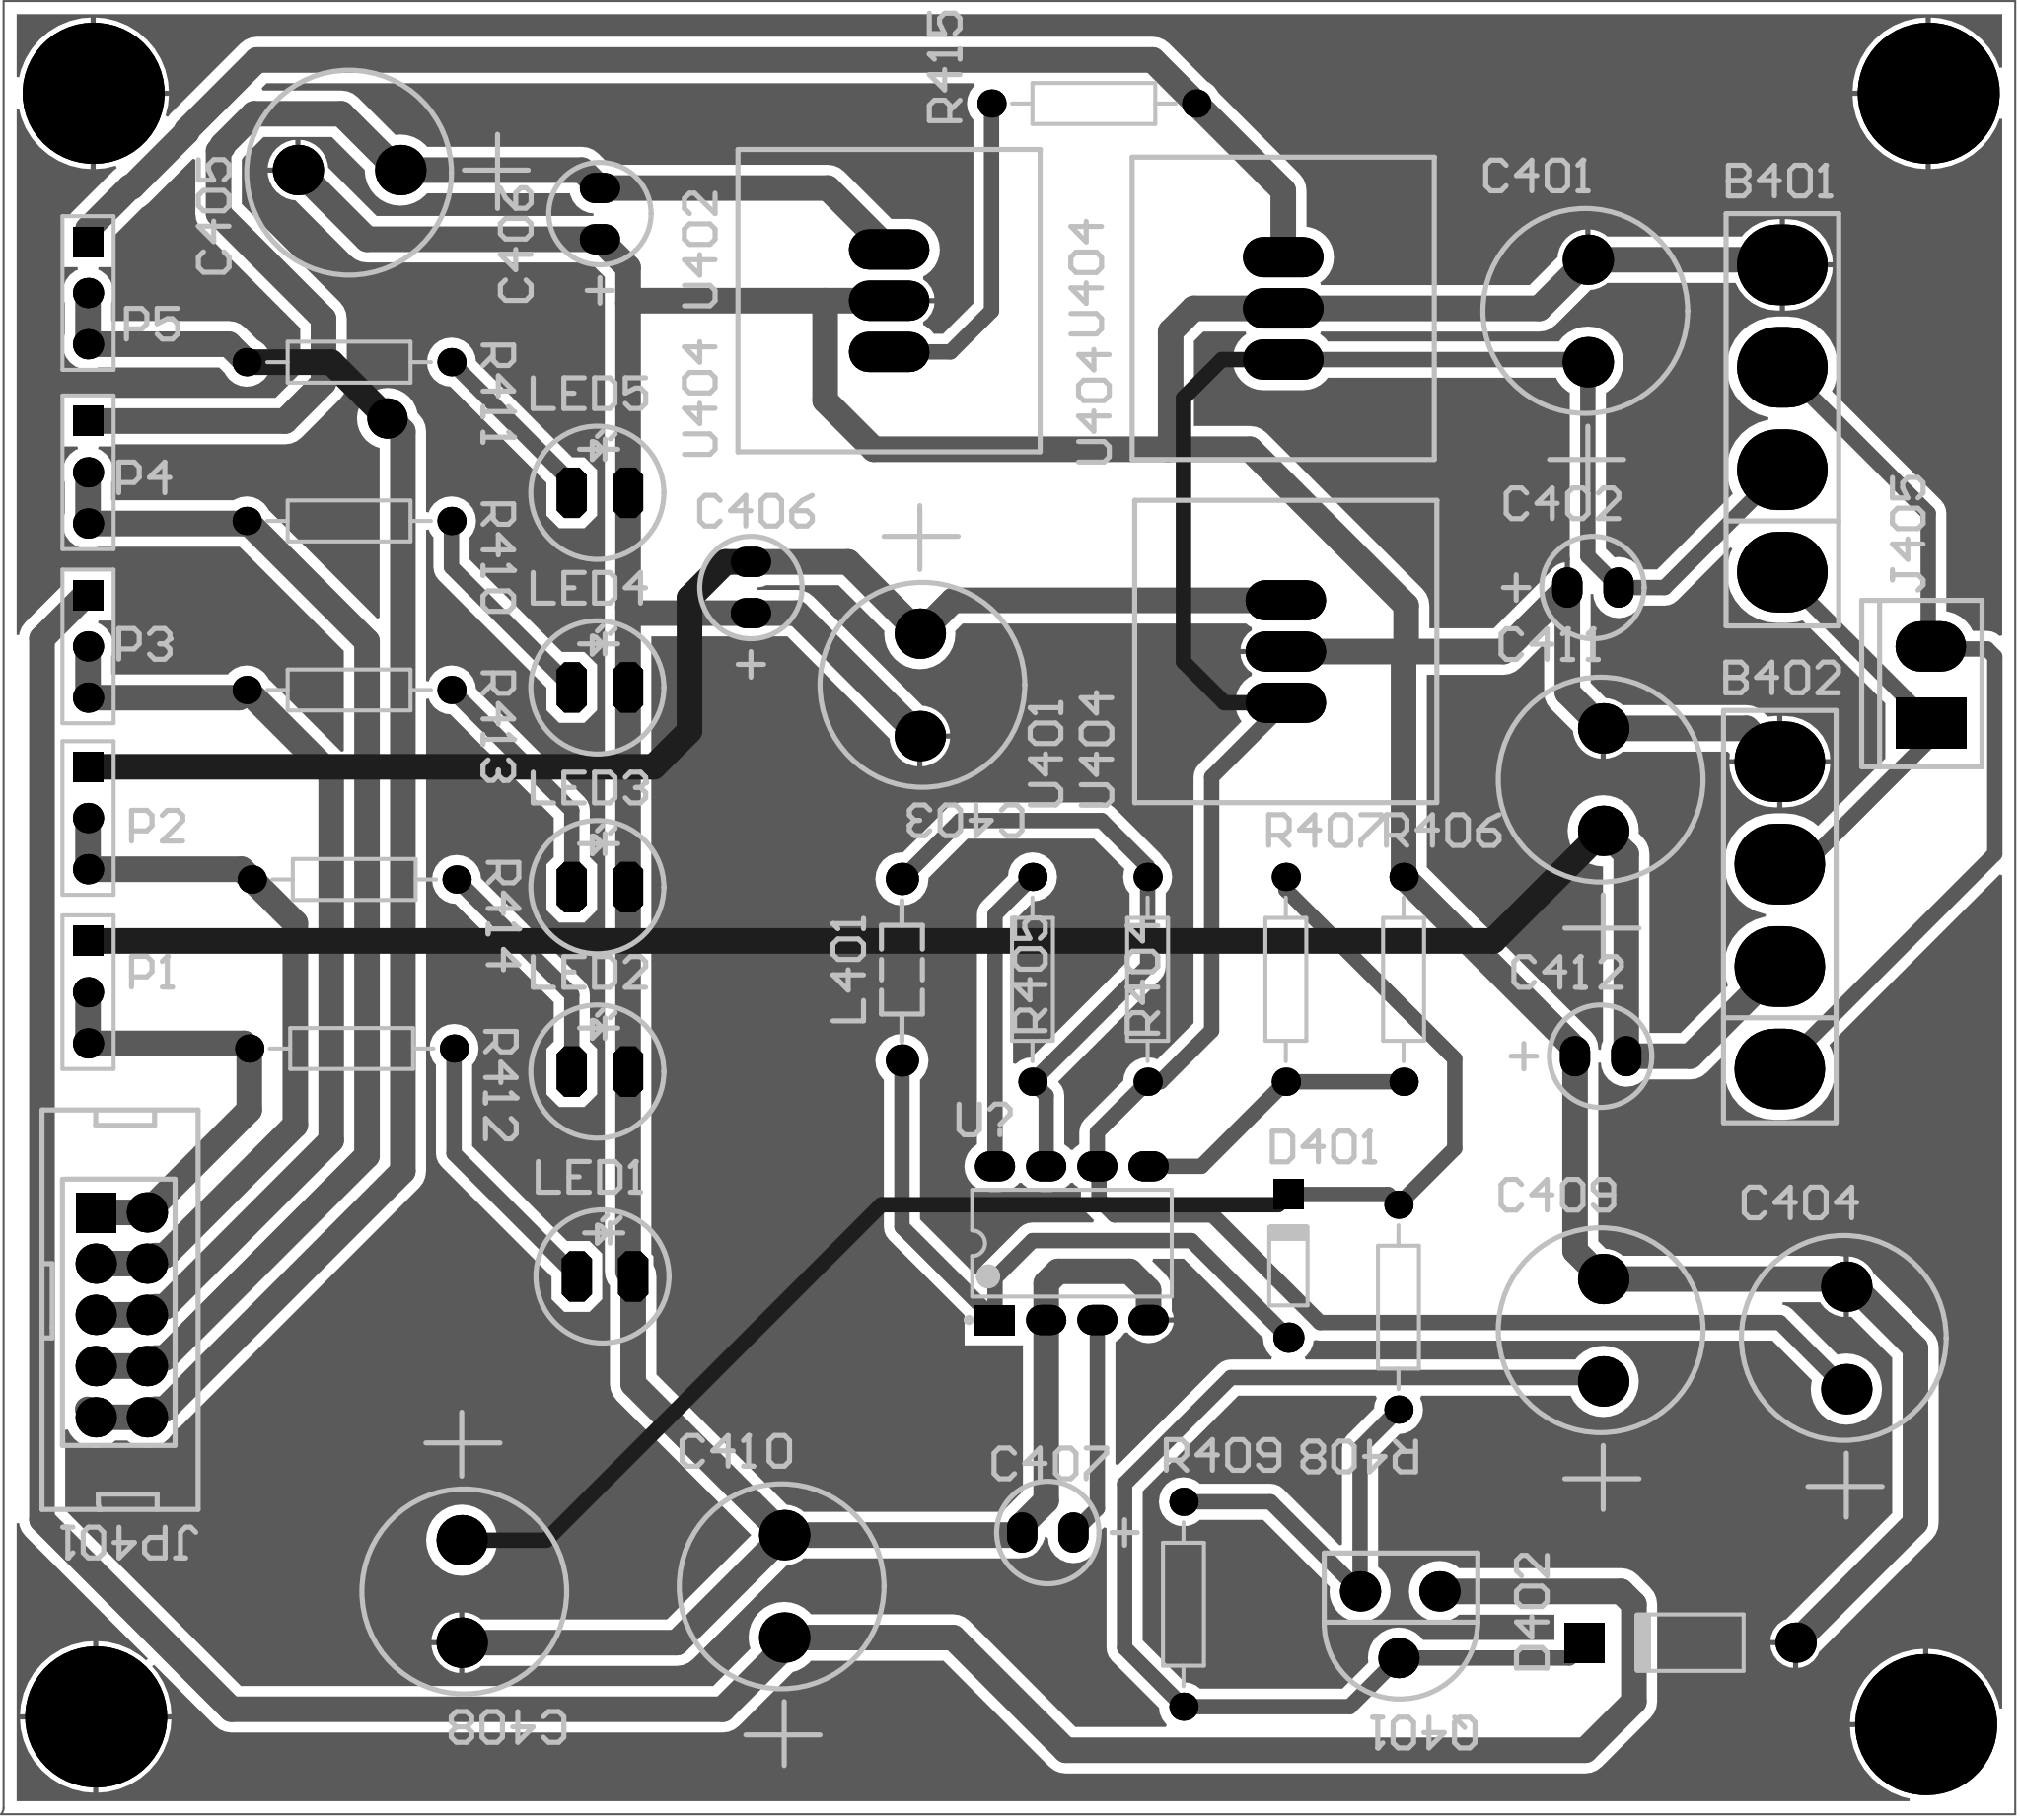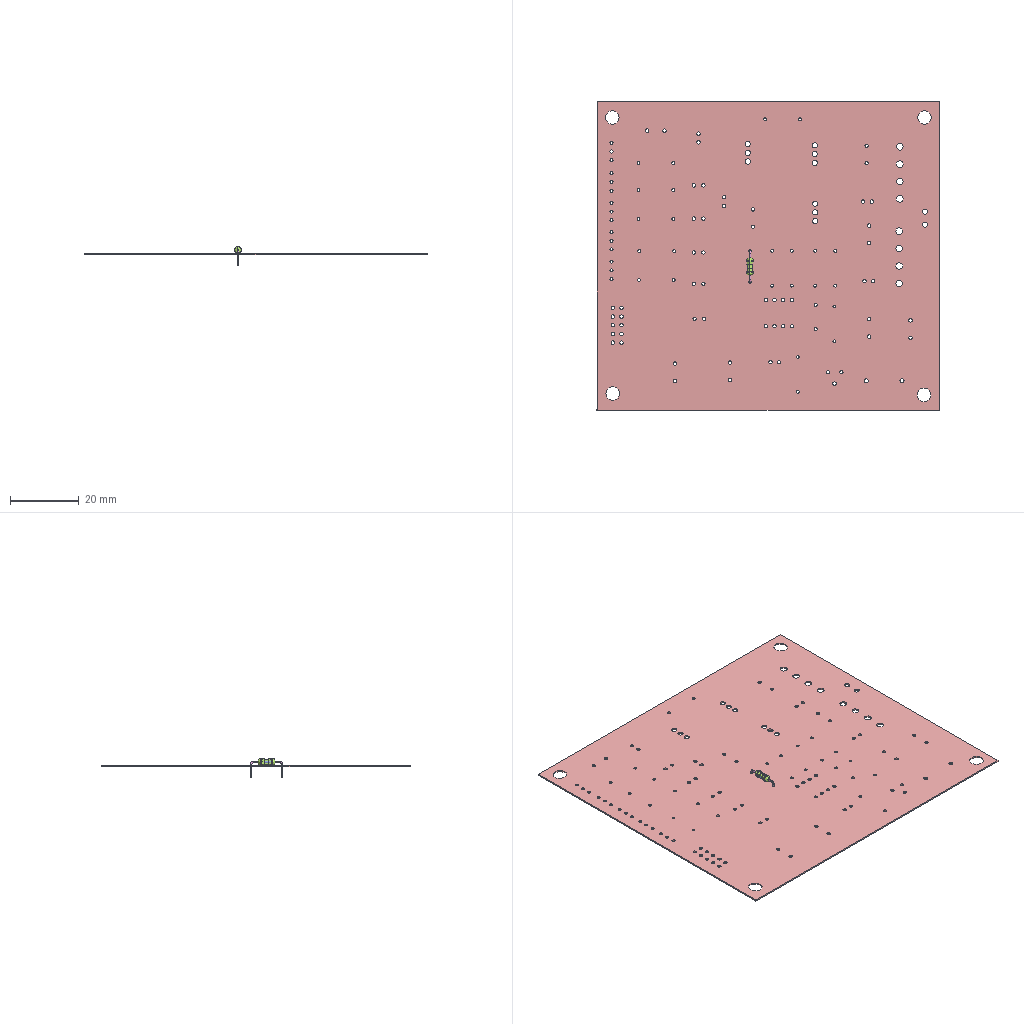Circuit board layout | Altium Designer | box 99.9 x 89.9 x 5.6 mm
Layer stack:
# Altium Designer layer stack of  (unit mm; dielectric type: 0 none, 1 core, 2 prepreg, 3 surface material)
index,name,kind,layer,copper_thickness_mm,dielectric_type,dielectric_thickness_mm,dielectric_material,dielectric_constant
0,Top Paste,other,,,,,,
1,Top Overlay,other,,,,,,
2,Top Solder,dielectric,,,3,0.0102,Solder Resist,3.5
3,Top Layer,copper,Top Layer,0.0356,,,,
4,Dielectric 1,dielectric,,,0,0.32,FR-4,4.8
5,Bottom Layer,copper,Bottom Layer,0.0356,,,,
6,Bottom Solder,dielectric,,,3,0.0102,Solder Resist,3.5
7,Bottom Overlay,other,,,,,,
8,Bottom Paste,other,,,,,,
# drill layer pairs: low layer,high layer
drill_pair,Top Layer,Bottom Layer
Part placement:
Designator,Comment,Layer,Footprint,Center-X(mm),Center-Y(mm),Rotation
U?,MC34063,TopLayer,MC34063,109.266,61.468,0
U404,7812,TopLayer,U404,119.761,107.823,90
U402,7805,TopLayer,U404,100.203,108.204,90
U401,7812,TopLayer,U404,119.888,90.805,90
R415,18/0.5W,TopLayer,AXIAL-0.4,110.363,117.983,180
R414,680,TopLayer,AXIAL-0.4,73.66,79.502,360
R413,15K,TopLayer,AXIAL-0.4,73.406,88.9,360
R412,1K,TopLayer,AXIAL-0.4,73.533,71.12,360
R411,680,TopLayer,AXIAL-0.4,73.406,105.156,360
R410,470,TopLayer,AXIAL-0.4,73.406,97.282,360
R409,1.5K,TopLayer,AXIAL-0.4,114.808,43.561,90
R408,47,TopLayer,AXIAL-0.4,125.476,58.293,270
R407,39K,TopLayer,AXIAL-0.4,119.888,74.549,90
R406,1.5K,TopLayer,AXIAL-0.4,125.73,74.549,90
R405,180,TopLayer,AXIAL-0.4,107.315,74.549,90
R404,2.2/1W,TopLayer,AXIAL-0.4,113.03,74.549,90
Q401,1815,TopLayer,Q401,125.54,42.545,180
P5,IFA12V,TopLayer,HDR1X3,60.452,108.585,270
P4,5V,TopLayer,HDR1X3,60.452,99.695,270
P3,33V,TopLayer,HDR1X3,60.452,91.059,270
P2,LCD12V,TopLayer,HDR1X3,60.452,82.55,270
P1,24V,TopLayer,HDR1X3,60.452,73.914,270
LED5,YELLOW,TopLayer,LED,85.852,98.679,0
LED4,WHITE,TopLayer,LED,85.852,89.027,0
LED3,BLUE,TopLayer,LED,85.852,79.121,360
LED2,GREEN,TopLayer,LED,85.852,69.977,0
LED1,RED,TopLayer,LED,86.106,59.817,0
L401,100UH/0.5W,TopLayer,AL0204,100.838,75.029,90
JP401,POWER,TopLayer,JP401,62.103,57.912,270
J405,AC18V,TopLayer,J405,151.892,89.154,90
D402,UPC574,TopLayer,DO-204AL,139.954,41.656,180
D401,4007,TopLayer,DO-35,120.015,60.331,90
C412,104,TopLayer,DR,135.509,70.739,0
C411,1000UF/50V,TopLayer,C401,135.636,84.455,90
C410,100UF/50V,TopLayer,C401,94.996,44.45,90
C409,100UF/50V,TopLayer,C401,135.636,57.15,90
C408,100UF/50V,TopLayer,C401,78.994,44.196,270
C407,152,TopLayer,DR,108.077,47.117,180
C406,104,TopLayer,DR,85.852,112.522,90
C406,104,TopLayer,DR,93.345,93.98,90
C405,47UF,TopLayer,C401,73.406,114.681,180
C404,100UF/50V,TopLayer,C401,147.701,56.769,90
C403,47UF,TopLayer,C401,101.727,89.154,270
C402,104,TopLayer,DR,135.128,93.98,360
C401,1000UF/50V,TopLayer,C401,134.874,107.696,90
B402,Bridge1,TopLayer,B401,144.399,77.724,90
B401,Bridge1,TopLayer,B401,144.526,102.362,90
Pad and via stacks:
# Altium Designer via and pad stacks of  (unit mm). Each distinct definition once, with the count of objects using it.
# via: kind,start_layer,end_layer,hole_mm,diameter_mm,mode(0 simple;1 top-mid-bottom;2 full stack),diameter_per_layer,count,example_net
# pad: kind,layer,hole_mm,hole_type(0 round;1 square;2 slot),plating,top_size,top_shape(1 round;2 rect;3 octagon;9 rounded rect),mid_size,bottom_size,mode,footprint,size_per_layer,count,example
pad,Multi-Layer,4,0,plated,7x7,1,7x7,7x7,0,,,4,3
pad,Multi-Layer,1,0,plated,2.5x2.5,1,2.5x2.5,2.5x2.5,0,C401,,16,C408.2
pad,Multi-Layer,0.85,0,plated,1.4x1.4,1,1.4x1.4,1.4x1.4,0,AXIAL-0.4,,24,R406.1
pad,Multi-Layer,0.9,0,plated,1.5x1.5,2,1.5x1.5,1.5x1.5,0,DO-35,,1,D401.2
pad,Multi-Layer,0.9,0,plated,1.5x1.5,1,1.5x1.5,1.5x1.5,0,DO-35,,1,D401.1
pad,Multi-Layer,1,0,plated,1.5x2,1,1.5x2,1.5x2,0,DR,,10,C407.1
pad,Multi-Layer,1,0,plated,2x2,1,2x2,2x2,0,Q401,,3,Q401.1
pad,Multi-Layer,0.8,0,plated,1.6x1.6,1,1.6x1.6,1.6x1.6,0,AL0204,,2,L401.2
pad,Multi-Layer,1,0,plated,2x1.5,2,2x1.5,2x1.5,0,MC34063,,1,U?.1
pad,Multi-Layer,1,0,plated,1.5x2,1,1.5x2,1.5x2,0,MC34063,,7,U?.2
pad,Multi-Layer,1.2,0,plated,2x2,1,2x2,2x2,0,DO-204AL,,1,D402.1
pad,Multi-Layer,1.2,0,plated,2x2,2,2x2,2x2,0,DO-204AL,,1,D402.2
pad,Multi-Layer,2,0,plated,4x4.5,1,4x4.5,4x4.5,0,B401,,8,B402.4
pad,Multi-Layer,1,0,plated,1.5x2.5,3,1.5x2.5,1.5x2.5,0,LED,,10,LED1.2
pad,Multi-Layer,1.5,0,plated,2x4,1,2x4,2x4,0,U404,,9,U402.1
pad,Multi-Layer,1.5,0,plated,2.5x3.5,2,2.5x3.5,2.5x3.5,0,J405,,1,J405.1
pad,Multi-Layer,1.5,0,plated,2.5x3.5,1,2.5x3.5,2.5x3.5,0,J405,,1,J405.2
pad,Multi-Layer,1,0,plated,2x2,2,2x2,2x2,0,JP401,,1,JP401.1
pad,Multi-Layer,1,0,plated,2x2,1,2x2,2x2,0,JP401,,9,JP401.3
pad,Multi-Layer,0.9,0,plated,1.5x1.5,2,1.5x1.5,1.5x1.5,0,HDR1X3,,5,P5.1
pad,Multi-Layer,0.9,0,plated,1.5x1.5,1,1.5x1.5,1.5x1.5,0,HDR1X3,,10,P5.2
via,Top Layer,Bottom Layer,1,2,0,,1,IFA12V
Copper pours:
name,layer,net,type(0 solid;1 hatched;2 none)
Top Layer-No Net,Bottom Layer,GND,0
Design rules, without the lines most boards share:
# Altium Designer design rules of  (exported by Altium Designer, unit mm)
# columns: name | kind | enabled | priority | scope1 | scope2 | descriptor | typed fields (field=value)
NetAntennae | 56 | enabled | 1 | All | All | Net Antennae (Tolerance=0mm) (All) |
SilkToSilkClearance | 55 | enabled | 1 | All | All | Silk to Silk (Clearance=0.254mm) (All),(All) |
SilkToSolderMaskClearance | 54 | enabled | 1 | IsPad | All | Silk To Solder Mask (Clearance=0.254mm) (IsPad),(All) |
MinimumSolderMaskSliver | 53 | enabled | 1 | All | All | Minimum Solder Mask Sliver (Gap=0.254mm) (All),(All) |
HoleToHoleClearance | 52 | enabled | 1 | All | All | Hole To Hole Clearance (Gap=0.254mm) (All),(All) | gap=0.254
DiffPairsRouting | 51 | enabled | 1 | All | All | Differential Pairs Uncoupled Length using the Gap Constraints (Min=0.254mm) (Max=0.254mm) (Prefered=0.254mm)  and Width Constraints (Min=0.381mm) (Max=0.381mm) (Prefered=0.381mm) (All) |
HoleSize | 42 | enabled | 1 | All | All | Hole Size Constraint (Min=0.025mm) (Max=2.54mm) (All) |
Height | 50 | enabled | 1 | All | All | Height Constraint (Min=0mm) (Max=25.4mm) (Prefered=12.7mm) (All) | min_height=0 max_height=25.4
ComponentClearance | 24 | enabled | 1 | All | All | Component Clearance Constraint ( Horizontal Gap = 0.254mm, Vertical Gap = 0.254mm ) (All),(All)  | gap=0.254
SolderMaskExpansion | 13 | enabled | 1 | All | All | Solder Mask Expansion (Expansion =0.102mm) (All) | expansion=0.1016
PasteMaskExpansion | 14 | enabled | 1 | All | All | Paste Mask Expansion (Expansion =0mm) (All) | expansion=0
RoutingVias | 11 | enabled | 1 | All | All | Routing Via (MinHoleWidth=0.711mm) (MaxHoleWidth=0.711mm) (PreferredHoleWidth=0.711mm) (MinWidth=1.27mm) (MaxWidth=1.27mm) (PreferedWidth=1.27mm) (All) | via_min_hole=0.7112 via_max_hole=0.7112 via_preferred_diameter=1.27 via_preferred_hole=0.7112
RoutingCorners | 10 | enabled | 1 | All | All | Routing Corners (Style=45-Degree) (Min Setback=2.54mm) (Max Setback=2.54mm) (All) |
Width | 2 | enabled | 1 | All | All | Width Constraint (Min=0.762mm) (Max=1.27mm) (Preferred=0.762mm) (All) |
PolygonConnect | 20 | enabled | 1 | All | All | Polygon Connect Rule(Relief Connect )(Conductor Width=0.254mm) (Relief Angle=90 Angle) (Entries=4) (Air Gap Width=0.254mm) (All),(All) | connect_style(0=relief,1=direct,2=none)=0 relief_conductor_width=0.254 relief_entries=4
PlaneClearance | 12 | enabled | 1 | All | All | Power Plane Clearance (Clearance =0.508mm) (All) | clearance=0.508
PlaneConnect | 6 | enabled | 1 | All | All | Power Plane Connect Rule(Relief Connect )(Expansion=0.508mm) (Conductor Width=0.254mm) (Air Gap=0.254mm) (Entries=4) (All) | relief_conductor_width=0.254 relief_entries=4 relief_expansion=0.508
Clearance | 0 | enabled | 1 | All | All | Clearance Constraint (Gap=0.508mm) (All),(All) | gap=0.508
Classes set for this board:
# Altium Designer classes of  (member kind: 0 net, 1 component, 2 from-to, 3 pad, 4 layer, 5 differential pair, 6 design channel, 7 polygon, 8 structure, 9 xSignal)
# columns: class name | member kind | superclass | members
Sheet1 | 1 | no | B401; B402; C401; C402; C403; C404; C405; C406; C406; C407; C408; C409; C410; C411; C412; D401; D402; J405; JP401; L401; LED1; LED2; LED3; LED4; LED5; P1; P2; P3; P4; P5; Q401; R404; R405; R406; R407; R408; R409; R410; R411; R412; R413; R414; R415; U401; U402; U404; U?;